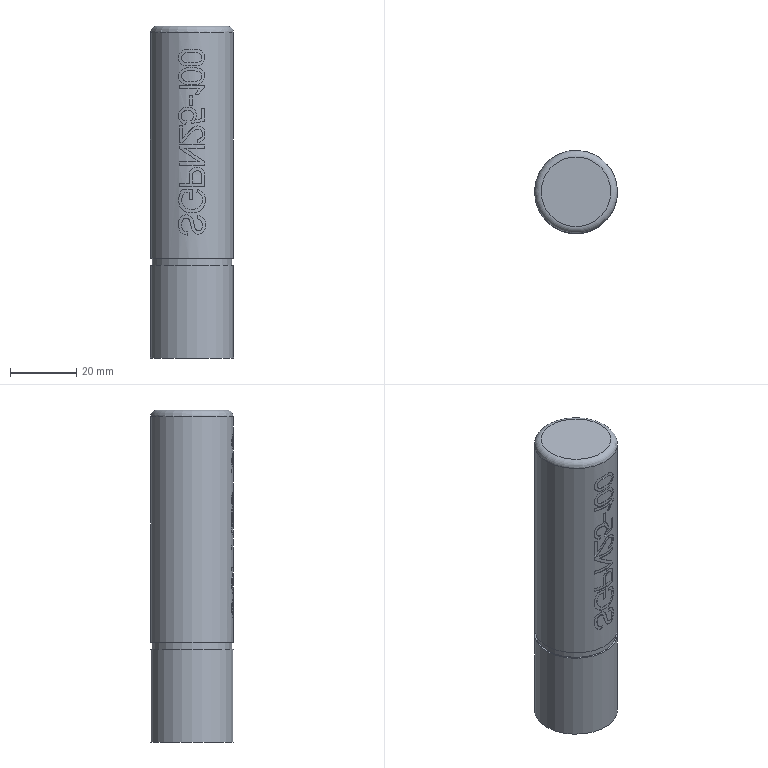Part | NX | features MI_SGPN_0291 2 | 1 solid | 152 faces | box 25 x 25 x 100 mm | volume 47826 mm3 | plane 83 | cylinder 66 | cone 2 | torus 1 | commonest cylinder face diameters 24.8 x10 25 x5 3.297 x2 3.934 x2 3.946 x2 3.992 x2